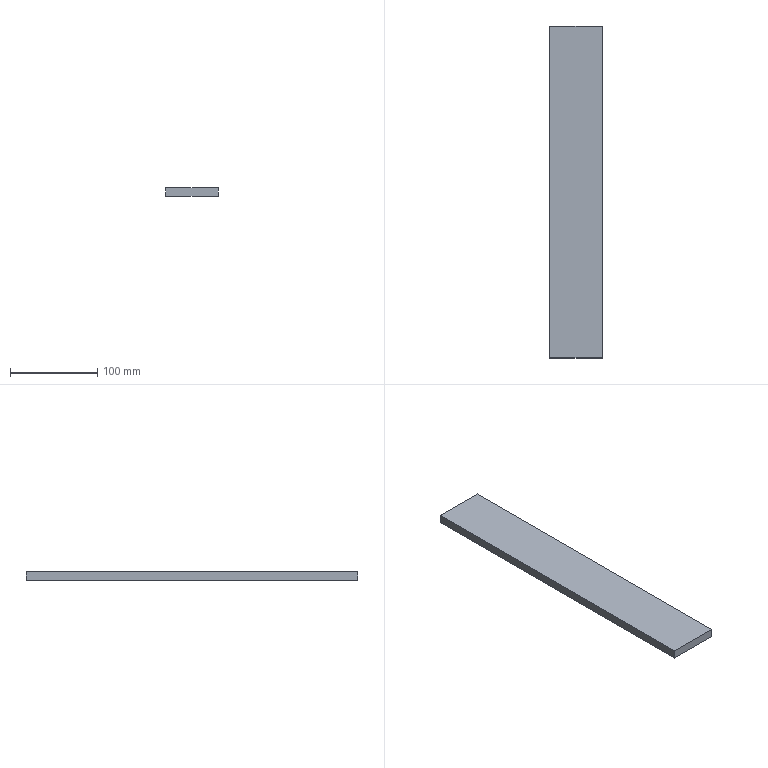Part | SolidWorks | features Extrusion 1 | 1 solid | 6 faces | box 60 x 380 x 10 mm | volume 228000 mm3 | plane 6
STEP:
#1=CARTESIAN_POINT('',(30.,-190.,0.));
#2=VERTEX_POINT('',#1);
#3=CARTESIAN_POINT('',(30.,190.,0.));
#4=VERTEX_POINT('',#3);
#5=CARTESIAN_POINT('',(30.,-190.,0.));
#6=DIRECTION('',(0.,1.,0.));
#7=VECTOR('',#6,1000.);
#8=LINE('',#5,#7);
#9=EDGE_CURVE('',#2,#4,#8,.T.);
#10=ORIENTED_EDGE('',*,*,#9,.T.);
#11=CARTESIAN_POINT('',(30.,190.,10.));
#12=VERTEX_POINT('',#11);
#13=CARTESIAN_POINT('',(30.,190.,10.));
#14=DIRECTION('',(0.,0.,-1.));
#15=VECTOR('',#14,1000.);
#16=LINE('',#13,#15);
#17=EDGE_CURVE('',#12,#4,#16,.T.);
#18=ORIENTED_EDGE('',*,*,#17,.F.);
#19=CARTESIAN_POINT('',(30.,-190.,10.));
#20=VERTEX_POINT('',#19);
#21=CARTESIAN_POINT('',(30.,-190.,10.));
#22=DIRECTION('',(0.,1.,0.));
#23=VECTOR('',#22,1000.);
#24=LINE('',#21,#23);
#25=EDGE_CURVE('',#20,#12,#24,.T.);
#26=ORIENTED_EDGE('',*,*,#25,.F.);
#27=CARTESIAN_POINT('',(30.,-190.,10.));
#28=DIRECTION('',(0.,0.,-1.));
#29=VECTOR('',#28,1000.);
#30=LINE('',#27,#29);
#31=EDGE_CURVE('',#20,#2,#30,.T.);
#32=ORIENTED_EDGE('',*,*,#31,.T.);
#33=EDGE_LOOP('',(#10,#18,#26,#32));
#34=FACE_OUTER_BOUND('',#33,.T.);
#35=CARTESIAN_POINT('',(30.,-190.,10.));
#36=DIRECTION('',(-1.,0.,0.));
#37=DIRECTION('',(0.,0.,1.));
#38=AXIS2_PLACEMENT_3D('',#35,#36,#37);
#39=PLANE('',#38);
#40=ADVANCED_FACE('',(#34),#39,.F.);
#41=CARTESIAN_POINT('',(-30.,190.,0.));
#42=VERTEX_POINT('',#41);
#43=CARTESIAN_POINT('',(-30.,190.,0.));
#44=DIRECTION('',(-1.,0.,0.));
#45=VECTOR('',#44,1000.);
#46=LINE('',#43,#45);
#47=EDGE_CURVE('',#4,#42,#46,.T.);
#48=ORIENTED_EDGE('',*,*,#47,.T.);
#49=CARTESIAN_POINT('',(-30.,190.,10.));
#50=VERTEX_POINT('',#49);
#51=CARTESIAN_POINT('',(-30.,190.,10.));
#52=DIRECTION('',(0.,0.,-1.));
#53=VECTOR('',#52,1000.);
#54=LINE('',#51,#53);
#55=EDGE_CURVE('',#50,#42,#54,.T.);
#56=ORIENTED_EDGE('',*,*,#55,.F.);
#57=CARTESIAN_POINT('',(-30.,190.,10.));
#58=DIRECTION('',(-1.,0.,0.));
#59=VECTOR('',#58,1000.);
#60=LINE('',#57,#59);
#61=EDGE_CURVE('',#12,#50,#60,.T.);
#62=ORIENTED_EDGE('',*,*,#61,.F.);
#63=ORIENTED_EDGE('',*,*,#17,.T.);
#64=EDGE_LOOP('',(#48,#56,#62,#63));
#65=FACE_OUTER_BOUND('',#64,.T.);
#66=CARTESIAN_POINT('',(-30.,190.,10.));
#67=DIRECTION('',(0.,-1.,0.));
#68=DIRECTION('',(0.,0.,-1.));
#69=AXIS2_PLACEMENT_3D('',#66,#67,#68);
#70=PLANE('',#69);
#71=ADVANCED_FACE('',(#65),#70,.F.);
#72=CARTESIAN_POINT('',(-30.,-190.,0.));
#73=VERTEX_POINT('',#72);
#74=CARTESIAN_POINT('',(-30.,-190.,0.));
#75=DIRECTION('',(0.,-1.,0.));
#76=VECTOR('',#75,1000.);
#77=LINE('',#74,#76);
#78=EDGE_CURVE('',#42,#73,#77,.T.);
#79=ORIENTED_EDGE('',*,*,#78,.T.);
#80=CARTESIAN_POINT('',(-30.,-190.,10.));
#81=VERTEX_POINT('',#80);
#82=CARTESIAN_POINT('',(-30.,-190.,10.));
#83=DIRECTION('',(0.,0.,-1.));
#84=VECTOR('',#83,1000.);
#85=LINE('',#82,#84);
#86=EDGE_CURVE('',#81,#73,#85,.T.);
#87=ORIENTED_EDGE('',*,*,#86,.F.);
#88=CARTESIAN_POINT('',(-30.,-190.,10.));
#89=DIRECTION('',(0.,-1.,0.));
#90=VECTOR('',#89,1000.);
#91=LINE('',#88,#90);
#92=EDGE_CURVE('',#50,#81,#91,.T.);
#93=ORIENTED_EDGE('',*,*,#92,.F.);
#94=ORIENTED_EDGE('',*,*,#55,.T.);
#95=EDGE_LOOP('',(#79,#87,#93,#94));
#96=FACE_OUTER_BOUND('',#95,.T.);
#97=CARTESIAN_POINT('',(-30.,-190.,10.));
#98=DIRECTION('',(1.,0.,0.));
#99=DIRECTION('',(0.,0.,-1.));
#100=AXIS2_PLACEMENT_3D('',#97,#98,#99);
#101=PLANE('',#100);
#102=ADVANCED_FACE('',(#96),#101,.F.);
#103=CARTESIAN_POINT('',(-30.,-190.,0.));
#104=DIRECTION('',(1.,0.,0.));
#105=VECTOR('',#104,1000.);
#106=LINE('',#103,#105);
#107=EDGE_CURVE('',#73,#2,#106,.T.);
#108=ORIENTED_EDGE('',*,*,#107,.T.);
#109=ORIENTED_EDGE('',*,*,#31,.F.);
#110=CARTESIAN_POINT('',(-30.,-190.,10.));
#111=DIRECTION('',(1.,0.,0.));
#112=VECTOR('',#111,1000.);
#113=LINE('',#110,#112);
#114=EDGE_CURVE('',#81,#20,#113,.T.);
#115=ORIENTED_EDGE('',*,*,#114,.F.);
#116=ORIENTED_EDGE('',*,*,#86,.T.);
#117=EDGE_LOOP('',(#108,#109,#115,#116));
#118=FACE_OUTER_BOUND('',#117,.T.);
#119=CARTESIAN_POINT('',(-30.,-190.,10.));
#120=DIRECTION('',(0.,1.,0.));
#121=DIRECTION('',(0.,0.,1.));
#122=AXIS2_PLACEMENT_3D('',#119,#120,#121);
#123=PLANE('',#122);
#124=ADVANCED_FACE('',(#118),#123,.F.);
#125=ORIENTED_EDGE('',*,*,#25,.T.);
#126=ORIENTED_EDGE('',*,*,#61,.T.);
#127=ORIENTED_EDGE('',*,*,#92,.T.);
#128=ORIENTED_EDGE('',*,*,#114,.T.);
#129=EDGE_LOOP('',(#125,#126,#127,#128));
#130=FACE_OUTER_BOUND('',#129,.T.);
#131=CARTESIAN_POINT('',(0.,0.,10.));
#132=DIRECTION('',(0.,0.,-1.));
#133=DIRECTION('',(-1.,0.,0.));
#134=AXIS2_PLACEMENT_3D('',#131,#132,#133);
#135=PLANE('',#134);
#136=ADVANCED_FACE('',(#130),#135,.F.);
#137=ORIENTED_EDGE('',*,*,#9,.F.);
#138=ORIENTED_EDGE('',*,*,#107,.F.);
#139=ORIENTED_EDGE('',*,*,#78,.F.);
#140=ORIENTED_EDGE('',*,*,#47,.F.);
#141=EDGE_LOOP('',(#137,#138,#139,#140));
#142=FACE_OUTER_BOUND('',#141,.T.);
#143=CARTESIAN_POINT('',(0.,0.,0.));
#144=DIRECTION('',(0.,0.,-1.));
#145=DIRECTION('',(-1.,0.,0.));
#146=AXIS2_PLACEMENT_3D('',#143,#144,#145);
#147=PLANE('',#146);
#148=ADVANCED_FACE('',(#142),#147,.T.);
#149=CLOSED_SHELL('',(#40,#71,#102,#124,#136,#148));
#150=MANIFOLD_SOLID_BREP('',#149);
#151=CARTESIAN_POINT('',(0.,0.,0.));
#152=DIRECTION('',(0.,0.,1.));
#153=DIRECTION('',(1.,0.,0.));
#154=AXIS2_PLACEMENT_3D('',#151,#152,#153);
#155=(LENGTH_UNIT()NAMED_UNIT(*)SI_UNIT(.MILLI.,.METRE.));
#156=UNCERTAINTY_MEASURE_WITH_UNIT(LENGTH_MEASURE(0.00001),#155,'','');
#157=(NAMED_UNIT(*)PLANE_ANGLE_UNIT()SI_UNIT($,.RADIAN.));
#158=(NAMED_UNIT(*)SI_UNIT($,.STERADIAN.)SOLID_ANGLE_UNIT());
#159=(GEOMETRIC_REPRESENTATION_CONTEXT(3)GLOBAL_UNCERTAINTY_ASSIGNED_CONTEXT((#156))GLOBAL_UNIT_ASSIGNED_CONTEXT((#155,#157,#158))REPRESENTATION_CONTEXT('',''));
#160=ADVANCED_BREP_SHAPE_REPRESENTATION('',(#150,#154),#159);